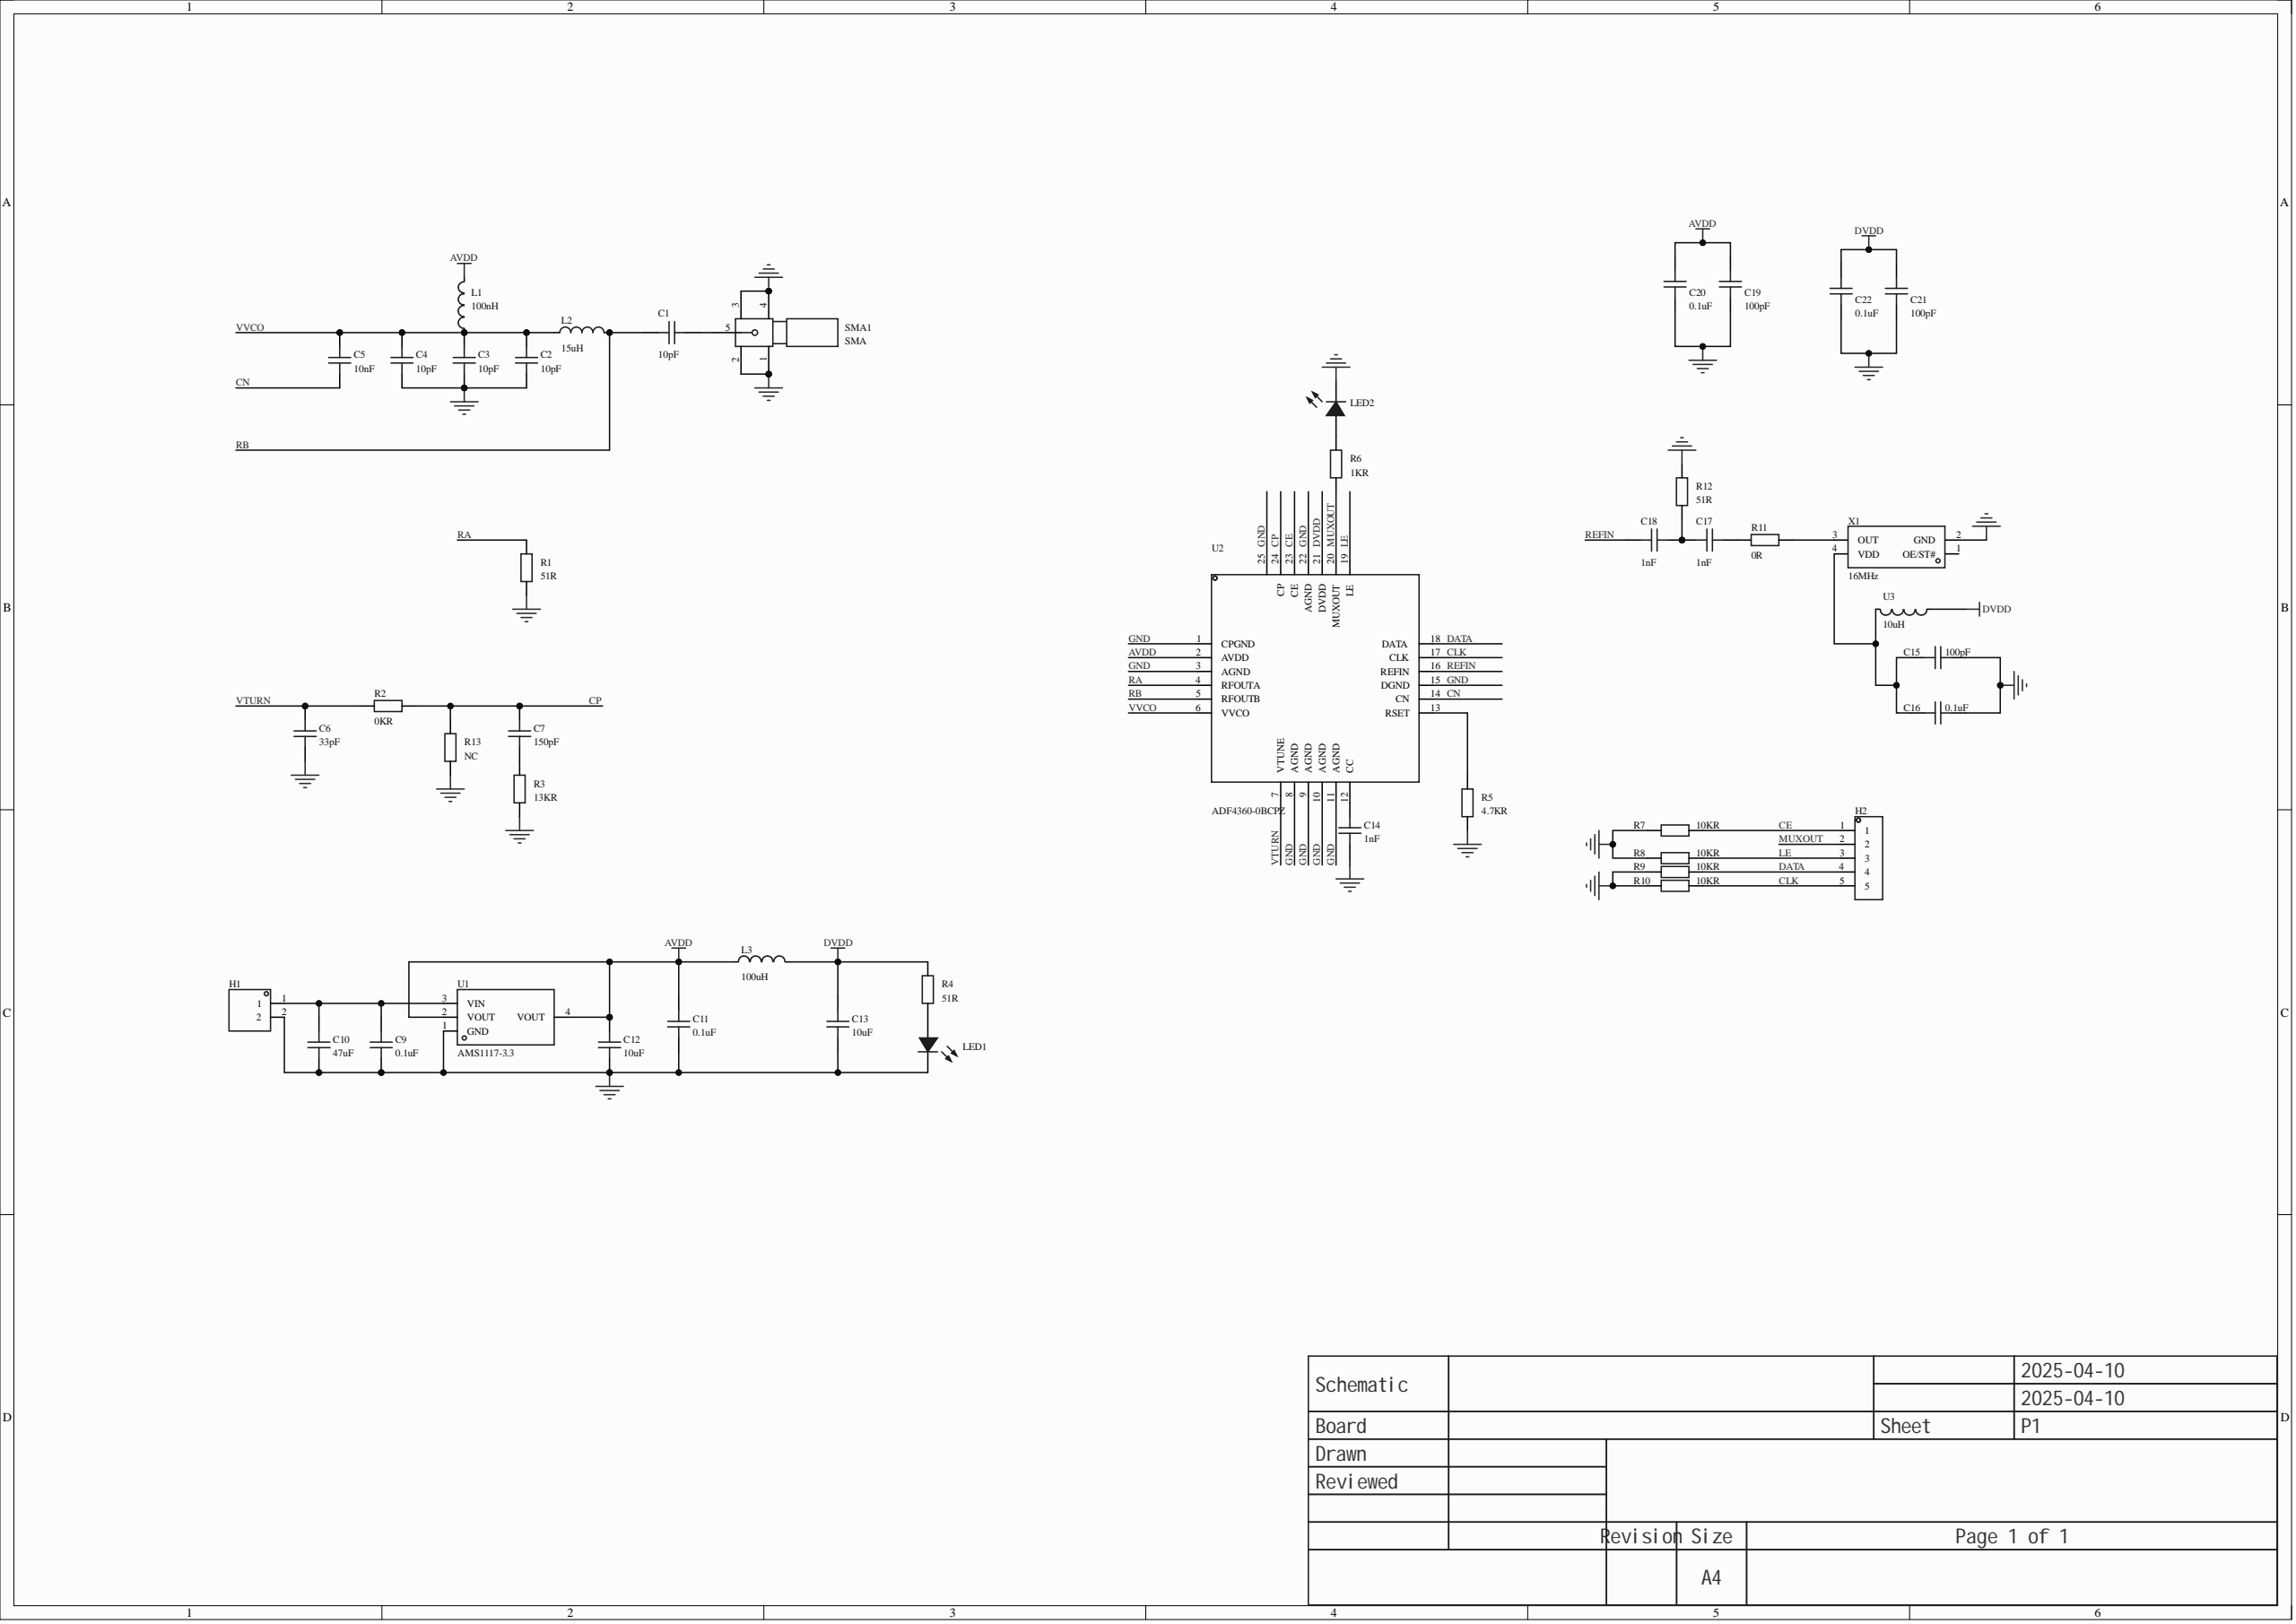Circuit board | Altium Designer | 46 parts | 26 nets
Bill of materials:
Comment,Description,Designator,Footprint,LibRef,Quantity
"10pF","","C1, C2, C3, C4","C0603","CAP_0603","4"
"10nF","","C5","C0603","CAP_0603","1"
"33pF","","C6","C0603","CAP_0603","1"
"150pF","","C7","C0603","CAP_0603","1"
"0.1uF","","C9, C11, C16, C20, C22","C0603","CAP_0603","5"
"47uF","","C10","C0603","CAP_0603","1"
"10uF","","C12, C13","C0603","CAP_0603","2"
"1nF","","C14, C17, C18","C0603","CAP_0603","3"
"100pF","","C15, C19, C21","C0603","CAP_0603","3"
"","","H1","HDR-TH_2P-P2.54-V-M-1","HDR-M_2.54_1x2P","1"
"","","H2","HDR-TH_5P-P2.54-V-M","HDR-M_2.54_1x5P","1"
"100nH","Inductance: 100nH; Tolerance: ±10%; Rated current: 250mA; Saturation current (Isat): -; DC resistance (DCR): 300mO;","L1","L0805","SDFL2012LR10KTF","1"
"15uH","Inductance: 15uH; Tolerance: ±20%; Rated current: 5A; Saturation current (Isat): 9A; Type: molded integrated inductor;","L2","IND-SMD_L8.5-W8.0-LS9.5_ZEYH0850-15UH","ZEYH0850-15UH","1"
"100uH","Inductance: 100uH; Tolerance: ±20%; Rated current: 250mA; Saturation current (Isat): 250mA; Type: -;","L3","IND-SMD_L4.0-W4.0_SWPA4018S","SWPA4012S101MT","1"
"","","LED1, LED2","LED_0603","LED_0603-B","2"
"51R","","R1, R4, R12","R0603","Res_0603","3"
"0KR","","R2","R0603","Res_0603","1"
"13KR","","R3","R0603","Res_0603","1"
"4.7KR","","R5","R0603","Res_0603","1"
"1KR","","R6","R0603","Res_0603","1"
"10KR","","R7, R8, R9, R10","R0603","Res_0603","4"
"0R","","R11","R0603","Res_0603","1"
"NC","","R13","R0603","Res_0603","1"
"SMA","","SMA1","SMA-SMD_BWSMA-KE-P001","SMA","1"
"AMS1117-3.3","Output type: fixed; Operating voltage: -; Output voltage: 3.3V; Output current: 1A; Power supply rejection ratio (PSRR): 72dB@(120Hz); Output polarity: positive;","U1","SOT-223-3_L6.5-W3.4-P2.30-LS7.0-BR","AMS1117-3.3_C6186","1"
"ADF4360-0BCPZ","Maximum output frequency: 2.725GHz;","U2","LFCSP-24_L4.0-W4.0-P0.50-BL-EP2.3","ADF4360-0BCPZ","1"
"10uH","","U3","IND-SMD_L4.0-W4.0_LVF404015","10uH","1"
"16MHz","Frequency: 16MHz; Frequency stability: ±100ppm; Operating voltage: 2.7V~3.6V;","X1","OSC-SMD_4P-L7.0-W5.0-BL","SG-8002CA 16MHz PCM","1"
Netlist (Protel format):
[
C1
C0603
10pF



]
[
C2
C0603
10pF



]
[
C3
C0603
10pF



]
[
C4
C0603
10pF



]
[
C5
C0603
10nF



]
[
C6
C0603
33pF



]
[
C7
C0603
150pF



]
[
C9
C0603
0.1uF



]
[
C10
C0603
47uF



]
[
C11
C0603
0.1uF



]
[
C12
C0603
10uF



]
[
C13
C0603
10uF



]
[
C14
C0603
1nF



]
[
C15
C0603
100pF



]
[
C16
C0603
0.1uF



]
[
C17
C0603
1nF



]
[
C18
C0603
1nF



]
[
C19
C0603
100pF



]
[
C20
C0603
0.1uF



]
[
C21
C0603
100pF



]
[
C22
C0603
0.1uF



]
[
H1
HDR-TH_2P-P2.54-V-M-1




]
[
H2
HDR-TH_5P-P2.54-V-M




]
[
L1
L0805
100nH



]
[
L2
IND-SMD_L8.5-W8.0-LS9.5_ZEYH0850-15UH
15uH



]
[
L3
IND-SMD_L4.0-W4.0_SWPA4018S
100uH



]
[
LED1
LED_0603




]
[
LED2
LED_0603




]
[
R1
R0603
51R



]
[
R2
R0603
0KR



]
[
R3
R0603
13KR



]
[
R4
R0603
51R



]
[
R5
R0603
4.7KR



]
[
R6
R0603
1KR



]
[
R7
R0603
10KR



]
[
R8
R0603
10KR



]
[
R9
R0603
10KR



]
[
R10
R0603
10KR



]
[
R11
R0603
0R



]
[
R12
R0603
51R



]
[
R13
R0603
NC



]
[
SMA1
SMA-SMD_BWSMA-KE-P001
SMA



]
[
U1
SOT-223-3_L6.5-W3.4-P2.30-LS7.0-BR
AMS1117-3.3



]
[
U2
LFCSP-24_L4.0-W4.0-P0.50-BL-EP2.3
ADF4360-0BCPZ



]
[
U3
IND-SMD_L4.0-W4.0_LVF404015
10uH



]
[
X1
OSC-SMD_4P-L7.0-W5.0-BL
16MHz



]
(
VVCO
C2-2
C3-2
C4-2
C5-2
L1-1
L2-1
U2-6
)
(
VTURN
C6-2
R2-2
U2-7
)
(
REFIN
C18-2
U2-16
)
(
RB
C1-1
L2-2
U2-5
)
(
RA
R1-2
U2-4
)
(
NetR11_2
R11-2
X1-3
)
(
NetR5_2
R5-2
U2-13
)
(
NetLED2_2
LED2-2
R6-1
)
(
NetLED1_2
LED1-2
R4-1
)
(
NetC17_2
C17-2
C18-1
R12-1
)
(
NetC17_1
C17-1
R11-1
)
(
NetC15_2
C15-2
C16-2
U3-2
X1-4
)
(
NetC14_2
C14-2
U2-12
)
(
NetC9_2
C9-2
C10-2
H1-1
U1-3
)
(
NetC7_1
C7-1
R3-1
)
(
NetC1_2
C1-2
SMA1-5
)
(
MUXOUT
H2-2
R6-2
U2-20
)
(
LE
H2-3
R8-1
U2-19
)
(
GND
C2-1
C3-1
C4-1
C6-1
C9-1
C10-1
C11-1
C12-1
C13-1
C14-1
C15-1
C16-1
C19-1
C20-1
C21-1
C22-1
H1-2
LED1-1
LED2-1
R1-1
R3-2
R5-1
R7-2
R8-2
R9-2
R10-2
R12-2
R13-2
SMA1-1
SMA1-2
SMA1-3
SMA1-4
U1-1
U2-1
U2-3
U2-8
U2-9
U2-10
U2-11
U2-15
U2-22
U2-25
X1-2
)
(
DVDD
C13-2
C21-2
C22-2
L3-2
R4-2
U2-21
U3-1
)
(
DATA
H2-4
R9-1
U2-18
)
(
CP
C7-2
R2-1
R13-1
U2-24
)
(
CN
C5-1
U2-14
)
(
CLK
H2-5
R10-1
U2-17
)
(
CE
H2-1
R7-1
U2-23
)
(
AVDD
C11-2
C12-2
C19-2
C20-2
L1-2
L3-1
U1-2
U1-4
U2-2
)